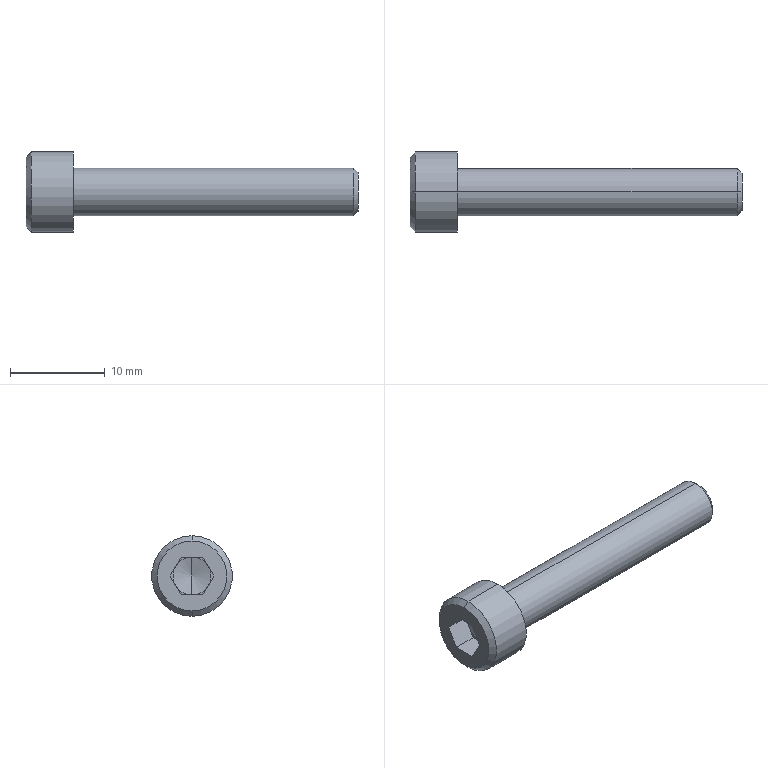Part | STEP file | 0246_310_SCB5-30 | 1 solid | 25 faces | box 35 x 8.5 x 8.5 mm | volume 830.025 mm3 | plane 15 | cone 6 | cylinder 4 | commonest cylinder face diameters 5 x2 8.5 x2